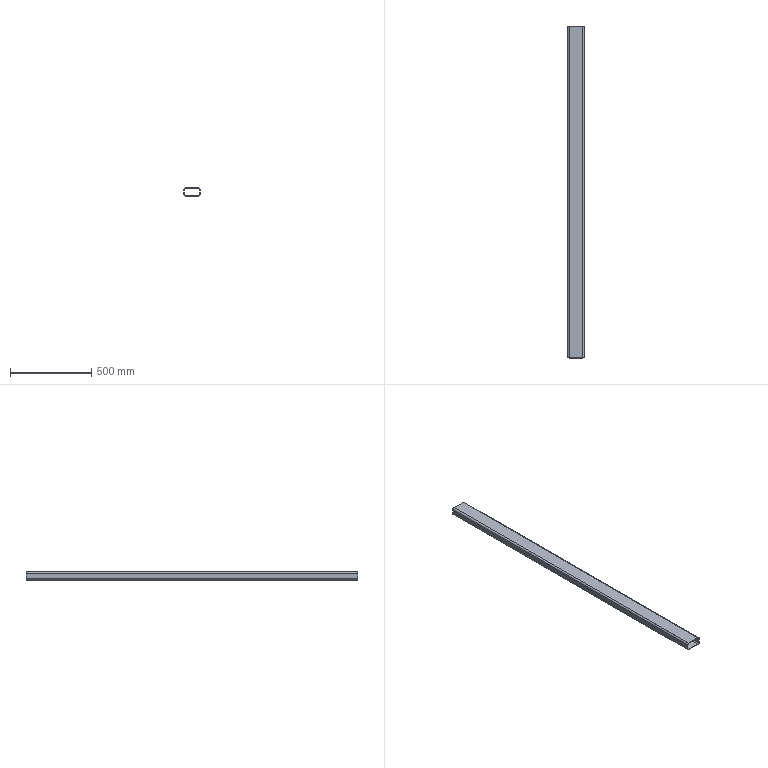Part | SolidWorks | features ExtruThin 1 | 1 solid | 18 faces | box 100 x 2040 x 50 mm | volume 1673251 mm3 | plane 10 | cylinder 8 | commonest cylinder face diameters 14 x4 20 x4
STEP:
#1=CARTESIAN_POINT('',(50.,1020.,-15.));
#2=VERTEX_POINT('',#1);
#3=CARTESIAN_POINT('',(40.,1020.,-25.));
#4=VERTEX_POINT('',#3);
#5=CARTESIAN_POINT('',(40.,1020.,-15.));
#6=DIRECTION('',(0.,1.,0.));
#7=DIRECTION('',(0.,0.,-1.));
#8=AXIS2_PLACEMENT_3D('',#5,#6,#7);
#9=CIRCLE('',#8,10.);
#10=EDGE_CURVE('',#2,#4,#9,.T.);
#11=ORIENTED_EDGE('',*,*,#10,.T.);
#12=CARTESIAN_POINT('',(-40.,1020.,-25.));
#13=VERTEX_POINT('',#12);
#14=CARTESIAN_POINT('',(-40.,1020.,-25.));
#15=DIRECTION('',(-1.,0.,0.));
#16=VECTOR('',#15,1000.);
#17=LINE('',#14,#16);
#18=EDGE_CURVE('',#4,#13,#17,.T.);
#19=ORIENTED_EDGE('',*,*,#18,.T.);
#20=CARTESIAN_POINT('',(-50.,1020.,-15.));
#21=VERTEX_POINT('',#20);
#22=CARTESIAN_POINT('',(-40.,1020.,-15.));
#23=DIRECTION('',(0.,1.,0.));
#24=DIRECTION('',(0.,0.,1.));
#25=AXIS2_PLACEMENT_3D('',#22,#23,#24);
#26=CIRCLE('',#25,10.);
#27=EDGE_CURVE('',#13,#21,#26,.T.);
#28=ORIENTED_EDGE('',*,*,#27,.T.);
#29=CARTESIAN_POINT('',(-50.,1020.,15.));
#30=VERTEX_POINT('',#29);
#31=CARTESIAN_POINT('',(-50.,1020.,-15.));
#32=DIRECTION('',(0.,0.,1.));
#33=VECTOR('',#32,1000.);
#34=LINE('',#31,#33);
#35=EDGE_CURVE('',#21,#30,#34,.T.);
#36=ORIENTED_EDGE('',*,*,#35,.T.);
#37=CARTESIAN_POINT('',(-40.,1020.,25.));
#38=VERTEX_POINT('',#37);
#39=CARTESIAN_POINT('',(-40.,1020.,15.));
#40=DIRECTION('',(0.,1.,0.));
#41=DIRECTION('',(0.,0.,1.));
#42=AXIS2_PLACEMENT_3D('',#39,#40,#41);
#43=CIRCLE('',#42,10.);
#44=EDGE_CURVE('',#30,#38,#43,.T.);
#45=ORIENTED_EDGE('',*,*,#44,.T.);
#46=CARTESIAN_POINT('',(40.,1020.,25.));
#47=VERTEX_POINT('',#46);
#48=CARTESIAN_POINT('',(-40.,1020.,25.));
#49=DIRECTION('',(1.,0.,0.));
#50=VECTOR('',#49,1000.);
#51=LINE('',#48,#50);
#52=EDGE_CURVE('',#38,#47,#51,.T.);
#53=ORIENTED_EDGE('',*,*,#52,.T.);
#54=CARTESIAN_POINT('',(50.,1020.,15.));
#55=VERTEX_POINT('',#54);
#56=CARTESIAN_POINT('',(40.,1020.,15.));
#57=DIRECTION('',(0.,1.,0.));
#58=DIRECTION('',(0.,0.,1.));
#59=AXIS2_PLACEMENT_3D('',#56,#57,#58);
#60=CIRCLE('',#59,10.);
#61=EDGE_CURVE('',#47,#55,#60,.T.);
#62=ORIENTED_EDGE('',*,*,#61,.T.);
#63=CARTESIAN_POINT('',(50.,1020.,-15.));
#64=DIRECTION('',(0.,0.,-1.));
#65=VECTOR('',#64,1000.);
#66=LINE('',#63,#65);
#67=EDGE_CURVE('',#55,#2,#66,.T.);
#68=ORIENTED_EDGE('',*,*,#67,.T.);
#69=EDGE_LOOP('',(#11,#19,#28,#36,#45,#53,#62,#68));
#70=FACE_OUTER_BOUND('',#69,.T.);
#71=CARTESIAN_POINT('',(40.,1020.,-22.));
#72=VERTEX_POINT('',#71);
#73=CARTESIAN_POINT('',(-40.,1020.,-22.));
#74=VERTEX_POINT('',#73);
#75=CARTESIAN_POINT('',(40.,1020.,-22.));
#76=DIRECTION('',(-1.,0.,0.));
#77=VECTOR('',#76,1000.);
#78=LINE('',#75,#77);
#79=EDGE_CURVE('',#72,#74,#78,.T.);
#80=ORIENTED_EDGE('',*,*,#79,.F.);
#81=CARTESIAN_POINT('',(47.,1020.,-15.));
#82=VERTEX_POINT('',#81);
#83=CARTESIAN_POINT('',(40.,1020.,-15.));
#84=DIRECTION('',(0.,1.,0.));
#85=DIRECTION('',(-1.,0.,0.));
#86=AXIS2_PLACEMENT_3D('',#83,#84,#85);
#87=CIRCLE('',#86,7.);
#88=EDGE_CURVE('',#82,#72,#87,.T.);
#89=ORIENTED_EDGE('',*,*,#88,.F.);
#90=CARTESIAN_POINT('',(47.,1020.,15.));
#91=VERTEX_POINT('',#90);
#92=CARTESIAN_POINT('',(47.,1020.,-15.));
#93=DIRECTION('',(0.,0.,-1.));
#94=VECTOR('',#93,1000.);
#95=LINE('',#92,#94);
#96=EDGE_CURVE('',#91,#82,#95,.T.);
#97=ORIENTED_EDGE('',*,*,#96,.F.);
#98=CARTESIAN_POINT('',(40.,1020.,22.));
#99=VERTEX_POINT('',#98);
#100=CARTESIAN_POINT('',(40.,1020.,15.));
#101=DIRECTION('',(0.,1.,0.));
#102=DIRECTION('',(-1.,0.,0.));
#103=AXIS2_PLACEMENT_3D('',#100,#101,#102);
#104=CIRCLE('',#103,7.);
#105=EDGE_CURVE('',#99,#91,#104,.T.);
#106=ORIENTED_EDGE('',*,*,#105,.F.);
#107=CARTESIAN_POINT('',(-40.,1020.,22.));
#108=VERTEX_POINT('',#107);
#109=CARTESIAN_POINT('',(40.,1020.,22.));
#110=DIRECTION('',(1.,0.,0.));
#111=VECTOR('',#110,1000.);
#112=LINE('',#109,#111);
#113=EDGE_CURVE('',#108,#99,#112,.T.);
#114=ORIENTED_EDGE('',*,*,#113,.F.);
#115=CARTESIAN_POINT('',(-47.,1020.,15.));
#116=VERTEX_POINT('',#115);
#117=CARTESIAN_POINT('',(-40.,1020.,15.));
#118=DIRECTION('',(0.,1.,0.));
#119=DIRECTION('',(-1.,0.,0.));
#120=AXIS2_PLACEMENT_3D('',#117,#118,#119);
#121=CIRCLE('',#120,7.);
#122=EDGE_CURVE('',#116,#108,#121,.T.);
#123=ORIENTED_EDGE('',*,*,#122,.F.);
#124=CARTESIAN_POINT('',(-47.,1020.,-15.));
#125=VERTEX_POINT('',#124);
#126=CARTESIAN_POINT('',(-47.,1020.,-15.));
#127=DIRECTION('',(0.,0.,1.));
#128=VECTOR('',#127,1000.);
#129=LINE('',#126,#128);
#130=EDGE_CURVE('',#125,#116,#129,.T.);
#131=ORIENTED_EDGE('',*,*,#130,.F.);
#132=CARTESIAN_POINT('',(-40.,1020.,-15.));
#133=DIRECTION('',(0.,1.,0.));
#134=DIRECTION('',(-1.,0.,0.));
#135=AXIS2_PLACEMENT_3D('',#132,#133,#134);
#136=CIRCLE('',#135,7.);
#137=EDGE_CURVE('',#74,#125,#136,.T.);
#138=ORIENTED_EDGE('',*,*,#137,.F.);
#139=EDGE_LOOP('',(#80,#89,#97,#106,#114,#123,#131,#138));
#140=FACE_BOUND('',#139,.T.);
#141=CARTESIAN_POINT('',(40.,1020.,-15.));
#142=DIRECTION('',(0.,1.,0.));
#143=DIRECTION('',(0.,0.,1.));
#144=AXIS2_PLACEMENT_3D('',#141,#142,#143);
#145=PLANE('',#144);
#146=ADVANCED_FACE('',(#70,#140),#145,.T.);
#147=CARTESIAN_POINT('',(50.,-1020.,-15.));
#148=VERTEX_POINT('',#147);
#149=CARTESIAN_POINT('',(40.,-1020.,-25.));
#150=VERTEX_POINT('',#149);
#151=CARTESIAN_POINT('',(40.,-1020.,-15.));
#152=DIRECTION('',(0.,1.,0.));
#153=DIRECTION('',(0.,0.,-1.));
#154=AXIS2_PLACEMENT_3D('',#151,#152,#153);
#155=CIRCLE('',#154,10.);
#156=EDGE_CURVE('',#148,#150,#155,.T.);
#157=ORIENTED_EDGE('',*,*,#156,.F.);
#158=CARTESIAN_POINT('',(50.,-1020.,15.));
#159=VERTEX_POINT('',#158);
#160=CARTESIAN_POINT('',(50.,-1020.,-15.));
#161=DIRECTION('',(0.,0.,-1.));
#162=VECTOR('',#161,1000.);
#163=LINE('',#160,#162);
#164=EDGE_CURVE('',#159,#148,#163,.T.);
#165=ORIENTED_EDGE('',*,*,#164,.F.);
#166=CARTESIAN_POINT('',(40.,-1020.,25.));
#167=VERTEX_POINT('',#166);
#168=CARTESIAN_POINT('',(40.,-1020.,15.));
#169=DIRECTION('',(0.,1.,0.));
#170=DIRECTION('',(0.,0.,1.));
#171=AXIS2_PLACEMENT_3D('',#168,#169,#170);
#172=CIRCLE('',#171,10.);
#173=EDGE_CURVE('',#167,#159,#172,.T.);
#174=ORIENTED_EDGE('',*,*,#173,.F.);
#175=CARTESIAN_POINT('',(-40.,-1020.,25.));
#176=VERTEX_POINT('',#175);
#177=CARTESIAN_POINT('',(-40.,-1020.,25.));
#178=DIRECTION('',(1.,0.,0.));
#179=VECTOR('',#178,1000.);
#180=LINE('',#177,#179);
#181=EDGE_CURVE('',#176,#167,#180,.T.);
#182=ORIENTED_EDGE('',*,*,#181,.F.);
#183=CARTESIAN_POINT('',(-50.,-1020.,15.));
#184=VERTEX_POINT('',#183);
#185=CARTESIAN_POINT('',(-40.,-1020.,15.));
#186=DIRECTION('',(0.,1.,0.));
#187=DIRECTION('',(0.,0.,1.));
#188=AXIS2_PLACEMENT_3D('',#185,#186,#187);
#189=CIRCLE('',#188,10.);
#190=EDGE_CURVE('',#184,#176,#189,.T.);
#191=ORIENTED_EDGE('',*,*,#190,.F.);
#192=CARTESIAN_POINT('',(-50.,-1020.,-15.));
#193=VERTEX_POINT('',#192);
#194=CARTESIAN_POINT('',(-50.,-1020.,-15.));
#195=DIRECTION('',(0.,0.,1.));
#196=VECTOR('',#195,1000.);
#197=LINE('',#194,#196);
#198=EDGE_CURVE('',#193,#184,#197,.T.);
#199=ORIENTED_EDGE('',*,*,#198,.F.);
#200=CARTESIAN_POINT('',(-40.,-1020.,-25.));
#201=VERTEX_POINT('',#200);
#202=CARTESIAN_POINT('',(-40.,-1020.,-15.));
#203=DIRECTION('',(0.,1.,0.));
#204=DIRECTION('',(0.,0.,1.));
#205=AXIS2_PLACEMENT_3D('',#202,#203,#204);
#206=CIRCLE('',#205,10.);
#207=EDGE_CURVE('',#201,#193,#206,.T.);
#208=ORIENTED_EDGE('',*,*,#207,.F.);
#209=CARTESIAN_POINT('',(-40.,-1020.,-25.));
#210=DIRECTION('',(-1.,0.,0.));
#211=VECTOR('',#210,1000.);
#212=LINE('',#209,#211);
#213=EDGE_CURVE('',#150,#201,#212,.T.);
#214=ORIENTED_EDGE('',*,*,#213,.F.);
#215=EDGE_LOOP('',(#157,#165,#174,#182,#191,#199,#208,#214));
#216=FACE_OUTER_BOUND('',#215,.T.);
#217=CARTESIAN_POINT('',(47.,-1020.,-15.));
#218=VERTEX_POINT('',#217);
#219=CARTESIAN_POINT('',(40.,-1020.,-22.));
#220=VERTEX_POINT('',#219);
#221=CARTESIAN_POINT('',(40.,-1020.,-15.));
#222=DIRECTION('',(0.,1.,0.));
#223=DIRECTION('',(-1.,0.,0.));
#224=AXIS2_PLACEMENT_3D('',#221,#222,#223);
#225=CIRCLE('',#224,7.);
#226=EDGE_CURVE('',#218,#220,#225,.T.);
#227=ORIENTED_EDGE('',*,*,#226,.T.);
#228=CARTESIAN_POINT('',(-40.,-1020.,-22.));
#229=VERTEX_POINT('',#228);
#230=CARTESIAN_POINT('',(40.,-1020.,-22.));
#231=DIRECTION('',(-1.,0.,0.));
#232=VECTOR('',#231,1000.);
#233=LINE('',#230,#232);
#234=EDGE_CURVE('',#220,#229,#233,.T.);
#235=ORIENTED_EDGE('',*,*,#234,.T.);
#236=CARTESIAN_POINT('',(-47.,-1020.,-15.));
#237=VERTEX_POINT('',#236);
#238=CARTESIAN_POINT('',(-40.,-1020.,-15.));
#239=DIRECTION('',(0.,1.,0.));
#240=DIRECTION('',(-1.,0.,0.));
#241=AXIS2_PLACEMENT_3D('',#238,#239,#240);
#242=CIRCLE('',#241,7.);
#243=EDGE_CURVE('',#229,#237,#242,.T.);
#244=ORIENTED_EDGE('',*,*,#243,.T.);
#245=CARTESIAN_POINT('',(-47.,-1020.,15.));
#246=VERTEX_POINT('',#245);
#247=CARTESIAN_POINT('',(-47.,-1020.,-15.));
#248=DIRECTION('',(0.,0.,1.));
#249=VECTOR('',#248,1000.);
#250=LINE('',#247,#249);
#251=EDGE_CURVE('',#237,#246,#250,.T.);
#252=ORIENTED_EDGE('',*,*,#251,.T.);
#253=CARTESIAN_POINT('',(-40.,-1020.,22.));
#254=VERTEX_POINT('',#253);
#255=CARTESIAN_POINT('',(-40.,-1020.,15.));
#256=DIRECTION('',(0.,1.,0.));
#257=DIRECTION('',(-1.,0.,0.));
#258=AXIS2_PLACEMENT_3D('',#255,#256,#257);
#259=CIRCLE('',#258,7.);
#260=EDGE_CURVE('',#246,#254,#259,.T.);
#261=ORIENTED_EDGE('',*,*,#260,.T.);
#262=CARTESIAN_POINT('',(40.,-1020.,22.));
#263=VERTEX_POINT('',#262);
#264=CARTESIAN_POINT('',(40.,-1020.,22.));
#265=DIRECTION('',(1.,0.,0.));
#266=VECTOR('',#265,1000.);
#267=LINE('',#264,#266);
#268=EDGE_CURVE('',#254,#263,#267,.T.);
#269=ORIENTED_EDGE('',*,*,#268,.T.);
#270=CARTESIAN_POINT('',(47.,-1020.,15.));
#271=VERTEX_POINT('',#270);
#272=CARTESIAN_POINT('',(40.,-1020.,15.));
#273=DIRECTION('',(0.,1.,0.));
#274=DIRECTION('',(-1.,0.,0.));
#275=AXIS2_PLACEMENT_3D('',#272,#273,#274);
#276=CIRCLE('',#275,7.);
#277=EDGE_CURVE('',#263,#271,#276,.T.);
#278=ORIENTED_EDGE('',*,*,#277,.T.);
#279=CARTESIAN_POINT('',(47.,-1020.,-15.));
#280=DIRECTION('',(0.,0.,-1.));
#281=VECTOR('',#280,1000.);
#282=LINE('',#279,#281);
#283=EDGE_CURVE('',#271,#218,#282,.T.);
#284=ORIENTED_EDGE('',*,*,#283,.T.);
#285=EDGE_LOOP('',(#227,#235,#244,#252,#261,#269,#278,#284));
#286=FACE_BOUND('',#285,.T.);
#287=CARTESIAN_POINT('',(40.,-1020.,-15.));
#288=DIRECTION('',(0.,1.,0.));
#289=DIRECTION('',(0.,0.,1.));
#290=AXIS2_PLACEMENT_3D('',#287,#288,#289);
#291=PLANE('',#290);
#292=ADVANCED_FACE('',(#216,#286),#291,.F.);
#293=ORIENTED_EDGE('',*,*,#156,.T.);
#294=CARTESIAN_POINT('',(40.,1020.,-25.));
#295=DIRECTION('',(0.,-1.,0.));
#296=VECTOR('',#295,1000.);
#297=LINE('',#294,#296);
#298=EDGE_CURVE('',#4,#150,#297,.T.);
#299=ORIENTED_EDGE('',*,*,#298,.F.);
#300=ORIENTED_EDGE('',*,*,#10,.F.);
#301=CARTESIAN_POINT('',(50.,1020.,-15.));
#302=DIRECTION('',(0.,-1.,0.));
#303=VECTOR('',#302,1000.);
#304=LINE('',#301,#303);
#305=EDGE_CURVE('',#2,#148,#304,.T.);
#306=ORIENTED_EDGE('',*,*,#305,.T.);
#307=EDGE_LOOP('',(#293,#299,#300,#306));
#308=FACE_OUTER_BOUND('',#307,.T.);
#309=CARTESIAN_POINT('',(40.,1020.,-15.));
#310=DIRECTION('',(0.,-1.,0.));
#311=DIRECTION('',(0.,0.,-1.));
#312=AXIS2_PLACEMENT_3D('',#309,#310,#311);
#313=CYLINDRICAL_SURFACE('',#312,10.);
#314=ADVANCED_FACE('',(#308),#313,.T.);
#315=ORIENTED_EDGE('',*,*,#213,.T.);
#316=CARTESIAN_POINT('',(-40.,1020.,-25.));
#317=DIRECTION('',(0.,-1.,0.));
#318=VECTOR('',#317,1000.);
#319=LINE('',#316,#318);
#320=EDGE_CURVE('',#13,#201,#319,.T.);
#321=ORIENTED_EDGE('',*,*,#320,.F.);
#322=ORIENTED_EDGE('',*,*,#18,.F.);
#323=ORIENTED_EDGE('',*,*,#298,.T.);
#324=EDGE_LOOP('',(#315,#321,#322,#323));
#325=FACE_OUTER_BOUND('',#324,.T.);
#326=CARTESIAN_POINT('',(-40.,1020.,-25.));
#327=DIRECTION('',(0.,0.,1.));
#328=DIRECTION('',(1.,0.,0.));
#329=AXIS2_PLACEMENT_3D('',#326,#327,#328);
#330=PLANE('',#329);
#331=ADVANCED_FACE('',(#325),#330,.F.);
#332=ORIENTED_EDGE('',*,*,#207,.T.);
#333=CARTESIAN_POINT('',(-50.,1020.,-15.));
#334=DIRECTION('',(0.,-1.,0.));
#335=VECTOR('',#334,1000.);
#336=LINE('',#333,#335);
#337=EDGE_CURVE('',#21,#193,#336,.T.);
#338=ORIENTED_EDGE('',*,*,#337,.F.);
#339=ORIENTED_EDGE('',*,*,#27,.F.);
#340=ORIENTED_EDGE('',*,*,#320,.T.);
#341=EDGE_LOOP('',(#332,#338,#339,#340));
#342=FACE_OUTER_BOUND('',#341,.T.);
#343=CARTESIAN_POINT('',(-40.,1020.,-15.));
#344=DIRECTION('',(0.,-1.,0.));
#345=DIRECTION('',(0.,0.,-1.));
#346=AXIS2_PLACEMENT_3D('',#343,#344,#345);
#347=CYLINDRICAL_SURFACE('',#346,10.);
#348=ADVANCED_FACE('',(#342),#347,.T.);
#349=ORIENTED_EDGE('',*,*,#198,.T.);
#350=CARTESIAN_POINT('',(-50.,1020.,15.));
#351=DIRECTION('',(0.,-1.,0.));
#352=VECTOR('',#351,1000.);
#353=LINE('',#350,#352);
#354=EDGE_CURVE('',#30,#184,#353,.T.);
#355=ORIENTED_EDGE('',*,*,#354,.F.);
#356=ORIENTED_EDGE('',*,*,#35,.F.);
#357=ORIENTED_EDGE('',*,*,#337,.T.);
#358=EDGE_LOOP('',(#349,#355,#356,#357));
#359=FACE_OUTER_BOUND('',#358,.T.);
#360=CARTESIAN_POINT('',(-50.,1020.,-15.));
#361=DIRECTION('',(1.,0.,0.));
#362=DIRECTION('',(0.,0.,-1.));
#363=AXIS2_PLACEMENT_3D('',#360,#361,#362);
#364=PLANE('',#363);
#365=ADVANCED_FACE('',(#359),#364,.F.);
#366=ORIENTED_EDGE('',*,*,#190,.T.);
#367=CARTESIAN_POINT('',(-40.,1020.,25.));
#368=DIRECTION('',(0.,-1.,0.));
#369=VECTOR('',#368,1000.);
#370=LINE('',#367,#369);
#371=EDGE_CURVE('',#38,#176,#370,.T.);
#372=ORIENTED_EDGE('',*,*,#371,.F.);
#373=ORIENTED_EDGE('',*,*,#44,.F.);
#374=ORIENTED_EDGE('',*,*,#354,.T.);
#375=EDGE_LOOP('',(#366,#372,#373,#374));
#376=FACE_OUTER_BOUND('',#375,.T.);
#377=CARTESIAN_POINT('',(-40.,1020.,15.));
#378=DIRECTION('',(0.,-1.,0.));
#379=DIRECTION('',(0.,0.,-1.));
#380=AXIS2_PLACEMENT_3D('',#377,#378,#379);
#381=CYLINDRICAL_SURFACE('',#380,10.);
#382=ADVANCED_FACE('',(#376),#381,.T.);
#383=ORIENTED_EDGE('',*,*,#181,.T.);
#384=CARTESIAN_POINT('',(40.,1020.,25.));
#385=DIRECTION('',(0.,-1.,0.));
#386=VECTOR('',#385,1000.);
#387=LINE('',#384,#386);
#388=EDGE_CURVE('',#47,#167,#387,.T.);
#389=ORIENTED_EDGE('',*,*,#388,.F.);
#390=ORIENTED_EDGE('',*,*,#52,.F.);
#391=ORIENTED_EDGE('',*,*,#371,.T.);
#392=EDGE_LOOP('',(#383,#389,#390,#391));
#393=FACE_OUTER_BOUND('',#392,.T.);
#394=CARTESIAN_POINT('',(-40.,1020.,25.));
#395=DIRECTION('',(0.,0.,-1.));
#396=DIRECTION('',(-1.,0.,0.));
#397=AXIS2_PLACEMENT_3D('',#394,#395,#396);
#398=PLANE('',#397);
#399=ADVANCED_FACE('',(#393),#398,.F.);
#400=ORIENTED_EDGE('',*,*,#173,.T.);
#401=CARTESIAN_POINT('',(50.,1020.,15.));
#402=DIRECTION('',(0.,-1.,0.));
#403=VECTOR('',#402,1000.);
#404=LINE('',#401,#403);
#405=EDGE_CURVE('',#55,#159,#404,.T.);
#406=ORIENTED_EDGE('',*,*,#405,.F.);
#407=ORIENTED_EDGE('',*,*,#61,.F.);
#408=ORIENTED_EDGE('',*,*,#388,.T.);
#409=EDGE_LOOP('',(#400,#406,#407,#408));
#410=FACE_OUTER_BOUND('',#409,.T.);
#411=CARTESIAN_POINT('',(40.,1020.,15.));
#412=DIRECTION('',(0.,-1.,0.));
#413=DIRECTION('',(0.,0.,-1.));
#414=AXIS2_PLACEMENT_3D('',#411,#412,#413);
#415=CYLINDRICAL_SURFACE('',#414,10.);
#416=ADVANCED_FACE('',(#410),#415,.T.);
#417=ORIENTED_EDGE('',*,*,#164,.T.);
#418=ORIENTED_EDGE('',*,*,#305,.F.);
#419=ORIENTED_EDGE('',*,*,#67,.F.);
#420=ORIENTED_EDGE('',*,*,#405,.T.);
#421=EDGE_LOOP('',(#417,#418,#419,#420));
#422=FACE_OUTER_BOUND('',#421,.T.);
#423=CARTESIAN_POINT('',(50.,1020.,-15.));
#424=DIRECTION('',(-1.,0.,0.));
#425=DIRECTION('',(0.,0.,1.));
#426=AXIS2_PLACEMENT_3D('',#423,#424,#425);
#427=PLANE('',#426);
#428=ADVANCED_FACE('',(#422),#427,.F.);
#429=ORIENTED_EDGE('',*,*,#226,.F.);
#430=CARTESIAN_POINT('',(47.,1020.,-15.));
#431=DIRECTION('',(0.,-1.,0.));
#432=VECTOR('',#431,1000.);
#433=LINE('',#430,#432);
#434=EDGE_CURVE('',#82,#218,#433,.T.);
#435=ORIENTED_EDGE('',*,*,#434,.F.);
#436=ORIENTED_EDGE('',*,*,#88,.T.);
#437=CARTESIAN_POINT('',(40.,1020.,-22.));
#438=DIRECTION('',(0.,-1.,0.));
#439=VECTOR('',#438,1000.);
#440=LINE('',#437,#439);
#441=EDGE_CURVE('',#72,#220,#440,.T.);
#442=ORIENTED_EDGE('',*,*,#441,.T.);
#443=EDGE_LOOP('',(#429,#435,#436,#442));
#444=FACE_OUTER_BOUND('',#443,.T.);
#445=CARTESIAN_POINT('',(40.,1020.,-15.));
#446=DIRECTION('',(0.,-1.,0.));
#447=DIRECTION('',(0.,0.,-1.));
#448=AXIS2_PLACEMENT_3D('',#445,#446,#447);
#449=CYLINDRICAL_SURFACE('',#448,7.);
#450=ADVANCED_FACE('',(#444),#449,.F.);
#451=ORIENTED_EDGE('',*,*,#234,.F.);
#452=ORIENTED_EDGE('',*,*,#441,.F.);
#453=ORIENTED_EDGE('',*,*,#79,.T.);
#454=CARTESIAN_POINT('',(-40.,1020.,-22.));
#455=DIRECTION('',(0.,-1.,0.));
#456=VECTOR('',#455,1000.);
#457=LINE('',#454,#456);
#458=EDGE_CURVE('',#74,#229,#457,.T.);
#459=ORIENTED_EDGE('',*,*,#458,.T.);
#460=EDGE_LOOP('',(#451,#452,#453,#459));
#461=FACE_OUTER_BOUND('',#460,.T.);
#462=CARTESIAN_POINT('',(40.,1020.,-22.));
#463=DIRECTION('',(0.,0.,1.));
#464=DIRECTION('',(1.,0.,0.));
#465=AXIS2_PLACEMENT_3D('',#462,#463,#464);
#466=PLANE('',#465);
#467=ADVANCED_FACE('',(#461),#466,.T.);
#468=ORIENTED_EDGE('',*,*,#243,.F.);
#469=ORIENTED_EDGE('',*,*,#458,.F.);
#470=ORIENTED_EDGE('',*,*,#137,.T.);
#471=CARTESIAN_POINT('',(-47.,1020.,-15.));
#472=DIRECTION('',(0.,-1.,0.));
#473=VECTOR('',#472,1000.);
#474=LINE('',#471,#473);
#475=EDGE_CURVE('',#125,#237,#474,.T.);
#476=ORIENTED_EDGE('',*,*,#475,.T.);
#477=EDGE_LOOP('',(#468,#469,#470,#476));
#478=FACE_OUTER_BOUND('',#477,.T.);
#479=CARTESIAN_POINT('',(-40.,1020.,-15.));
#480=DIRECTION('',(0.,-1.,0.));
#481=DIRECTION('',(0.,0.,-1.));
#482=AXIS2_PLACEMENT_3D('',#479,#480,#481);
#483=CYLINDRICAL_SURFACE('',#482,7.);
#484=ADVANCED_FACE('',(#478),#483,.F.);
#485=ORIENTED_EDGE('',*,*,#251,.F.);
#486=ORIENTED_EDGE('',*,*,#475,.F.);
#487=ORIENTED_EDGE('',*,*,#130,.T.);
#488=CARTESIAN_POINT('',(-47.,1020.,15.));
#489=DIRECTION('',(0.,-1.,0.));
#490=VECTOR('',#489,1000.);
#491=LINE('',#488,#490);
#492=EDGE_CURVE('',#116,#246,#491,.T.);
#493=ORIENTED_EDGE('',*,*,#492,.T.);
#494=EDGE_LOOP('',(#485,#486,#487,#493));
#495=FACE_OUTER_BOUND('',#494,.T.);
#496=CARTESIAN_POINT('',(-47.,1020.,-15.));
#497=DIRECTION('',(1.,0.,0.));
#498=DIRECTION('',(0.,0.,-1.));
#499=AXIS2_PLACEMENT_3D('',#496,#497,#498);
#500=PLANE('',#499);
#501=ADVANCED_FACE('',(#495),#500,.T.);
#502=ORIENTED_EDGE('',*,*,#260,.F.);
#503=ORIENTED_EDGE('',*,*,#492,.F.);
#504=ORIENTED_EDGE('',*,*,#122,.T.);
#505=CARTESIAN_POINT('',(-40.,1020.,22.));
#506=DIRECTION('',(0.,-1.,0.));
#507=VECTOR('',#506,1000.);
#508=LINE('',#505,#507);
#509=EDGE_CURVE('',#108,#254,#508,.T.);
#510=ORIENTED_EDGE('',*,*,#509,.T.);
#511=EDGE_LOOP('',(#502,#503,#504,#510));
#512=FACE_OUTER_BOUND('',#511,.T.);
#513=CARTESIAN_POINT('',(-40.,1020.,15.));
#514=DIRECTION('',(0.,-1.,0.));
#515=DIRECTION('',(0.,0.,-1.));
#516=AXIS2_PLACEMENT_3D('',#513,#514,#515);
#517=CYLINDRICAL_SURFACE('',#516,7.);
#518=ADVANCED_FACE('',(#512),#517,.F.);
#519=ORIENTED_EDGE('',*,*,#268,.F.);
#520=ORIENTED_EDGE('',*,*,#509,.F.);
#521=ORIENTED_EDGE('',*,*,#113,.T.);
#522=CARTESIAN_POINT('',(40.,1020.,22.));
#523=DIRECTION('',(0.,-1.,0.));
#524=VECTOR('',#523,1000.);
#525=LINE('',#522,#524);
#526=EDGE_CURVE('',#99,#263,#525,.T.);
#527=ORIENTED_EDGE('',*,*,#526,.T.);
#528=EDGE_LOOP('',(#519,#520,#521,#527));
#529=FACE_OUTER_BOUND('',#528,.T.);
#530=CARTESIAN_POINT('',(40.,1020.,22.));
#531=DIRECTION('',(0.,0.,-1.));
#532=DIRECTION('',(-1.,0.,0.));
#533=AXIS2_PLACEMENT_3D('',#530,#531,#532);
#534=PLANE('',#533);
#535=ADVANCED_FACE('',(#529),#534,.T.);
#536=ORIENTED_EDGE('',*,*,#277,.F.);
#537=ORIENTED_EDGE('',*,*,#526,.F.);
#538=ORIENTED_EDGE('',*,*,#105,.T.);
#539=CARTESIAN_POINT('',(47.,1020.,15.));
#540=DIRECTION('',(0.,-1.,0.));
#541=VECTOR('',#540,1000.);
#542=LINE('',#539,#541);
#543=EDGE_CURVE('',#91,#271,#542,.T.);
#544=ORIENTED_EDGE('',*,*,#543,.T.);
#545=EDGE_LOOP('',(#536,#537,#538,#544));
#546=FACE_OUTER_BOUND('',#545,.T.);
#547=CARTESIAN_POINT('',(40.,1020.,15.));
#548=DIRECTION('',(0.,-1.,0.));
#549=DIRECTION('',(0.,0.,-1.));
#550=AXIS2_PLACEMENT_3D('',#547,#548,#549);
#551=CYLINDRICAL_SURFACE('',#550,7.);
#552=ADVANCED_FACE('',(#546),#551,.F.);
#553=ORIENTED_EDGE('',*,*,#283,.F.);
#554=ORIENTED_EDGE('',*,*,#543,.F.);
#555=ORIENTED_EDGE('',*,*,#96,.T.);
#556=ORIENTED_EDGE('',*,*,#434,.T.);
#557=EDGE_LOOP('',(#553,#554,#555,#556));
#558=FACE_OUTER_BOUND('',#557,.T.);
#559=CARTESIAN_POINT('',(47.,1020.,-15.));
#560=DIRECTION('',(-1.,0.,0.));
#561=DIRECTION('',(0.,0.,1.));
#562=AXIS2_PLACEMENT_3D('',#559,#560,#561);
#563=PLANE('',#562);
#564=ADVANCED_FACE('',(#558),#563,.T.);
#565=CLOSED_SHELL('',(#146,#292,#314,#331,#348,#365,#382,#399,#416,#428,#450,#467,#484,#501,#518,#535,#552,#564));
#566=MANIFOLD_SOLID_BREP('',#565);
#567=CARTESIAN_POINT('',(0.,0.,0.));
#568=DIRECTION('',(0.,0.,1.));
#569=DIRECTION('',(1.,0.,0.));
#570=AXIS2_PLACEMENT_3D('',#567,#568,#569);
#571=(LENGTH_UNIT()NAMED_UNIT(*)SI_UNIT(.MILLI.,.METRE.));
#572=UNCERTAINTY_MEASURE_WITH_UNIT(LENGTH_MEASURE(0.00001),#571,'','');
#573=(NAMED_UNIT(*)PLANE_ANGLE_UNIT()SI_UNIT($,.RADIAN.));
#574=(NAMED_UNIT(*)SI_UNIT($,.STERADIAN.)SOLID_ANGLE_UNIT());
#575=(GEOMETRIC_REPRESENTATION_CONTEXT(3)GLOBAL_UNCERTAINTY_ASSIGNED_CONTEXT((#572))GLOBAL_UNIT_ASSIGNED_CONTEXT((#571,#573,#574))REPRESENTATION_CONTEXT('',''));
#576=ADVANCED_BREP_SHAPE_REPRESENTATION('',(#566,#570),#575);